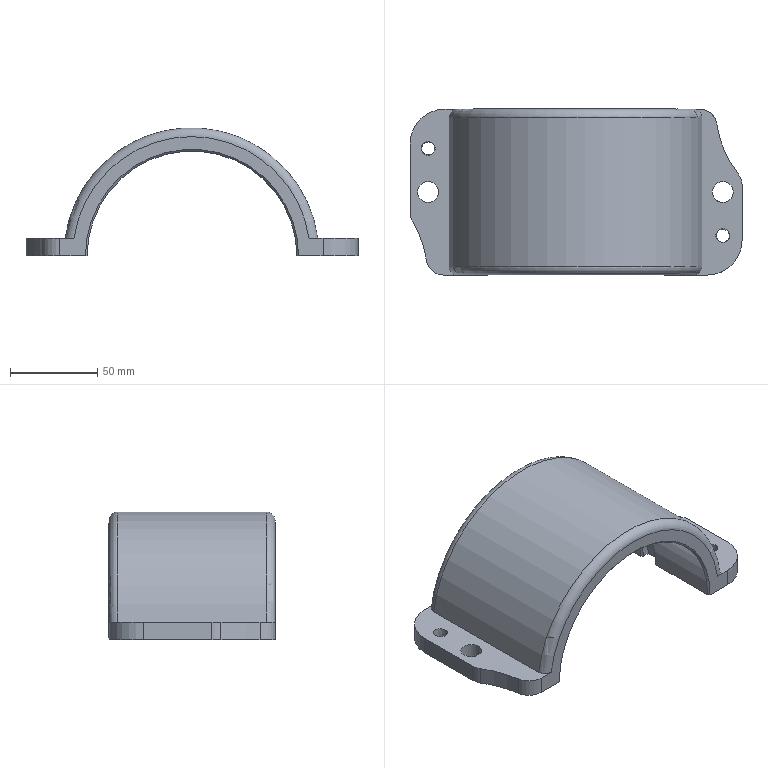Part | NX | features BREP 1, CHAMFER 1, DATUM_CSYS 1, DATUM_PLANE 1 | 1 solid | 32 faces | box 190 x 95 x 73.244 mm | volume 279574 mm3 | cylinder 14 | plane 10 | cone 6 | torus 2 | commonest cylinder face diameters 20 x4 120 x4 12 x2 40 x2 130 x1 146 x1
STEP:
#1=CARTESIAN_POINT('',(240.308,-695.5,40.));
#2=VERTEX_POINT('',#1);
#3=CARTESIAN_POINT('',(244.046,-695.5,40.));
#4=DIRECTION('',(0.,0.,-1.));
#5=DIRECTION('',(-1.,0.,0.));
#6=AXIS2_PLACEMENT_3D('',#3,#4,#5);
#7=CIRCLE('',#6,3.738);
#8=EDGE_CURVE('',#2,#2,#7,.F.);
#9=ORIENTED_EDGE('',*,*,#8,.T.);
#10=EDGE_LOOP('',(#9));
#11=FACE_BOUND('',#10,.T.);
#12=CARTESIAN_POINT('',(238.046,-670.5,40.));
#13=VERTEX_POINT('',#12);
#14=CARTESIAN_POINT('',(244.046,-670.5,40.));
#15=DIRECTION('',(0.,0.,-1.));
#16=DIRECTION('',(-1.,0.,0.));
#17=AXIS2_PLACEMENT_3D('',#14,#15,#16);
#18=CIRCLE('',#17,6.);
#19=EDGE_CURVE('',#13,#13,#18,.F.);
#20=ORIENTED_EDGE('',*,*,#19,.T.);
#21=EDGE_LOOP('',(#20));
#22=FACE_BOUND('',#21,.T.);
#23=CARTESIAN_POINT('',(220.,-624.,40.));
#24=VERTEX_POINT('',#23);
#25=CARTESIAN_POINT('',(220.,-663.,40.));
#26=VERTEX_POINT('',#25);
#27=CARTESIAN_POINT('',(220.,-611.,40.));
#28=DIRECTION('',(0.,-1.,0.));
#29=VECTOR('',#28,1000.);
#30=LINE('',#27,#29);
#31=EDGE_CURVE('',#24,#26,#30,.T.);
#32=ORIENTED_EDGE('',*,*,#31,.F.);
#33=CARTESIAN_POINT('',(221.,-623.,40.));
#34=VERTEX_POINT('',#33);
#35=CARTESIAN_POINT('',(160.,-684.,40.));
#36=DIRECTION('',(-0.7071,-0.7071,0.));
#37=VECTOR('',#36,1000.);
#38=LINE('',#35,#37);
#39=EDGE_CURVE('',#24,#34,#38,.F.);
#40=ORIENTED_EDGE('',*,*,#39,.T.);
#41=CARTESIAN_POINT('',(227.701,-623.,40.));
#42=VERTEX_POINT('',#41);
#43=CARTESIAN_POINT('',(85.,-623.,40.));
#44=DIRECTION('',(1.,0.,0.));
#45=VECTOR('',#44,1000.);
#46=LINE('',#43,#45);
#47=EDGE_CURVE('',#34,#42,#46,.T.);
#48=ORIENTED_EDGE('',*,*,#47,.T.);
#49=CARTESIAN_POINT('',(228.948,-623.158,40.));
#50=VERTEX_POINT('',#49);
#51=CARTESIAN_POINT('',(227.701,-623.,40.));
#52=CARTESIAN_POINT('',(228.123,-623.,40.));
#53=CARTESIAN_POINT('',(228.539,-623.053,40.));
#54=CARTESIAN_POINT('',(228.948,-623.158,40.));
#55=B_SPLINE_CURVE_WITH_KNOTS('',3,(#51,#52,#53,#54),.UNSPECIFIED.,.F.,.F.,(4,4),(0.,0.001257),.UNSPECIFIED.);
#56=EDGE_CURVE('',#42,#50,#55,.T.);
#57=ORIENTED_EDGE('',*,*,#56,.T.);
#58=CARTESIAN_POINT('',(240.615,-631.571,40.));
#59=VERTEX_POINT('',#58);
#60=CARTESIAN_POINT('',(230.718,-633.,40.));
#61=DIRECTION('',(0.,0.,-1.));
#62=DIRECTION('',(-1.,0.,0.));
#63=AXIS2_PLACEMENT_3D('',#60,#61,#62);
#64=CIRCLE('',#63,10.);
#65=EDGE_CURVE('',#50,#59,#64,.T.);
#66=ORIENTED_EDGE('',*,*,#65,.T.);
#67=CARTESIAN_POINT('',(252.857,-660.115,40.));
#68=VERTEX_POINT('',#67);
#69=CARTESIAN_POINT('',(300.,-623.,40.));
#70=DIRECTION('',(0.,0.,1.));
#71=DIRECTION('',(-1.,0.,0.));
#72=AXIS2_PLACEMENT_3D('',#69,#70,#71);
#73=CIRCLE('',#72,60.);
#74=EDGE_CURVE('',#59,#68,#73,.T.);
#75=ORIENTED_EDGE('',*,*,#74,.T.);
#76=CARTESIAN_POINT('',(255.,-666.301,40.));
#77=VERTEX_POINT('',#76);
#78=CARTESIAN_POINT('',(245.,-666.301,40.));
#79=DIRECTION('',(0.,0.,-1.));
#80=DIRECTION('',(-1.,0.,0.));
#81=AXIS2_PLACEMENT_3D('',#78,#79,#80);
#82=CIRCLE('',#81,10.);
#83=EDGE_CURVE('',#68,#77,#82,.T.);
#84=ORIENTED_EDGE('',*,*,#83,.T.);
#85=CARTESIAN_POINT('',(255.,-698.,40.));
#86=VERTEX_POINT('',#85);
#87=CARTESIAN_POINT('',(255.,-662.686,40.));
#88=DIRECTION('',(0.,-1.,0.));
#89=VECTOR('',#88,1000.);
#90=LINE('',#87,#89);
#91=EDGE_CURVE('',#77,#86,#90,.T.);
#92=ORIENTED_EDGE('',*,*,#91,.T.);
#93=CARTESIAN_POINT('',(235.,-718.,40.));
#94=VERTEX_POINT('',#93);
#95=CARTESIAN_POINT('',(235.,-698.,40.));
#96=DIRECTION('',(0.,0.,-1.));
#97=DIRECTION('',(-1.,0.,0.));
#98=AXIS2_PLACEMENT_3D('',#95,#96,#97);
#99=CIRCLE('',#98,20.);
#100=EDGE_CURVE('',#86,#94,#99,.T.);
#101=ORIENTED_EDGE('',*,*,#100,.T.);
#102=CARTESIAN_POINT('',(221.,-718.,40.));
#103=VERTEX_POINT('',#102);
#104=CARTESIAN_POINT('',(235.,-718.,40.));
#105=DIRECTION('',(-1.,0.,0.));
#106=VECTOR('',#105,1000.);
#107=LINE('',#104,#106);
#108=EDGE_CURVE('',#94,#103,#107,.T.);
#109=ORIENTED_EDGE('',*,*,#108,.T.);
#110=CARTESIAN_POINT('',(220.,-717.,40.));
#111=VERTEX_POINT('',#110);
#112=CARTESIAN_POINT('',(160.,-657.,40.));
#113=DIRECTION('',(0.7071,-0.7071,0.));
#114=VECTOR('',#113,1000.);
#115=LINE('',#112,#114);
#116=EDGE_CURVE('',#103,#111,#115,.F.);
#117=ORIENTED_EDGE('',*,*,#116,.T.);
#118=CARTESIAN_POINT('',(220.,-675.,40.));
#119=VERTEX_POINT('',#118);
#120=CARTESIAN_POINT('',(220.,-611.,40.));
#121=DIRECTION('',(0.,-1.,0.));
#122=VECTOR('',#121,1000.);
#123=LINE('',#120,#122);
#124=EDGE_CURVE('',#119,#111,#123,.T.);
#125=ORIENTED_EDGE('',*,*,#124,.F.);
#126=CARTESIAN_POINT('',(221.,-674.,40.));
#127=VERTEX_POINT('',#126);
#128=CARTESIAN_POINT('',(160.,-735.,40.));
#129=DIRECTION('',(-0.7071,-0.7071,0.));
#130=VECTOR('',#129,1000.);
#131=LINE('',#128,#130);
#132=EDGE_CURVE('',#119,#127,#131,.F.);
#133=ORIENTED_EDGE('',*,*,#132,.T.);
#134=CARTESIAN_POINT('',(225.,-674.,40.));
#135=VERTEX_POINT('',#134);
#136=CARTESIAN_POINT('',(85.,-674.,40.));
#137=DIRECTION('',(1.,0.,0.));
#138=VECTOR('',#137,1000.);
#139=LINE('',#136,#138);
#140=EDGE_CURVE('',#127,#135,#139,.T.);
#141=ORIENTED_EDGE('',*,*,#140,.T.);
#142=CARTESIAN_POINT('',(225.,-664.,40.));
#143=VERTEX_POINT('',#142);
#144=CARTESIAN_POINT('',(225.,-664.,40.));
#145=DIRECTION('',(0.,-1.,0.));
#146=VECTOR('',#145,1000.);
#147=LINE('',#144,#146);
#148=EDGE_CURVE('',#135,#143,#147,.F.);
#149=ORIENTED_EDGE('',*,*,#148,.T.);
#150=CARTESIAN_POINT('',(221.,-664.,40.));
#151=VERTEX_POINT('',#150);
#152=CARTESIAN_POINT('',(85.,-664.,40.));
#153=DIRECTION('',(1.,0.,0.));
#154=VECTOR('',#153,1000.);
#155=LINE('',#152,#154);
#156=EDGE_CURVE('',#151,#143,#155,.T.);
#157=ORIENTED_EDGE('',*,*,#156,.F.);
#158=CARTESIAN_POINT('',(160.,-603.,40.));
#159=DIRECTION('',(0.7071,-0.7071,0.));
#160=VECTOR('',#159,1000.);
#161=LINE('',#158,#160);
#162=EDGE_CURVE('',#151,#26,#161,.F.);
#163=ORIENTED_EDGE('',*,*,#162,.T.);
#164=EDGE_LOOP('',(#32,#40,#48,#57,#66,#75,#84,#92,#101,#109,#117,#125,#133,#141,#149,#157,#163));
#165=FACE_BOUND('',#164,.T.);
#166=CARTESIAN_POINT('',(85.,-643.,40.));
#167=DIRECTION('',(0.,0.,-1.));
#168=DIRECTION('',(-1.,0.,0.));
#169=AXIS2_PLACEMENT_3D('',#166,#167,#168);
#170=PLANE('',#169);
#171=ADVANCED_FACE('',(#11,#22,#165),#170,.T.);
#172=CARTESIAN_POINT('',(244.046,-691.5,50.));
#173=VERTEX_POINT('',#172);
#174=CARTESIAN_POINT('',(244.046,-695.5,50.));
#175=DIRECTION('',(0.,0.,-1.));
#176=DIRECTION('',(0.,1.,0.));
#177=AXIS2_PLACEMENT_3D('',#174,#175,#176);
#178=CIRCLE('',#177,4.);
#179=EDGE_CURVE('',#173,#173,#178,.T.);
#180=ORIENTED_EDGE('',*,*,#179,.T.);
#181=EDGE_LOOP('',(#180));
#182=FACE_BOUND('',#181,.T.);
#183=CARTESIAN_POINT('',(244.046,-664.5,50.));
#184=VERTEX_POINT('',#183);
#185=CARTESIAN_POINT('',(244.046,-670.5,50.));
#186=DIRECTION('',(0.,0.,-1.));
#187=DIRECTION('',(0.,1.,0.));
#188=AXIS2_PLACEMENT_3D('',#185,#186,#187);
#189=CIRCLE('',#188,6.);
#190=EDGE_CURVE('',#184,#184,#189,.T.);
#191=ORIENTED_EDGE('',*,*,#190,.T.);
#192=EDGE_LOOP('',(#191));
#193=FACE_BOUND('',#192,.T.);
#194=CARTESIAN_POINT('',(255.,-666.301,50.));
#195=VERTEX_POINT('',#194);
#196=CARTESIAN_POINT('',(255.,-698.,50.));
#197=VERTEX_POINT('',#196);
#198=CARTESIAN_POINT('',(255.,-662.686,50.));
#199=DIRECTION('',(0.,-1.,0.));
#200=VECTOR('',#199,1000.);
#201=LINE('',#198,#200);
#202=EDGE_CURVE('',#195,#197,#201,.T.);
#203=ORIENTED_EDGE('',*,*,#202,.F.);
#204=CARTESIAN_POINT('',(252.857,-660.115,50.));
#205=VERTEX_POINT('',#204);
#206=CARTESIAN_POINT('',(245.,-666.301,50.));
#207=DIRECTION('',(0.,0.,-1.));
#208=DIRECTION('',(-1.,0.,0.));
#209=AXIS2_PLACEMENT_3D('',#206,#207,#208);
#210=CIRCLE('',#209,10.);
#211=EDGE_CURVE('',#195,#205,#210,.F.);
#212=ORIENTED_EDGE('',*,*,#211,.T.);
#213=CARTESIAN_POINT('',(240.615,-631.571,50.));
#214=VERTEX_POINT('',#213);
#215=CARTESIAN_POINT('',(300.,-623.,50.));
#216=DIRECTION('',(0.,0.,1.));
#217=DIRECTION('',(-1.,0.,0.));
#218=AXIS2_PLACEMENT_3D('',#215,#216,#217);
#219=CIRCLE('',#218,60.);
#220=EDGE_CURVE('',#214,#205,#219,.T.);
#221=ORIENTED_EDGE('',*,*,#220,.F.);
#222=CARTESIAN_POINT('',(228.542,-623.24,50.));
#223=VERTEX_POINT('',#222);
#224=CARTESIAN_POINT('',(230.718,-633.,50.));
#225=DIRECTION('',(0.,0.,-1.));
#226=DIRECTION('',(-1.,0.,0.));
#227=AXIS2_PLACEMENT_3D('',#224,#225,#226);
#228=CIRCLE('',#227,10.);
#229=EDGE_CURVE('',#214,#223,#228,.F.);
#230=ORIENTED_EDGE('',*,*,#229,.T.);
#231=CARTESIAN_POINT('',(232.046,-628.,50.));
#232=VERTEX_POINT('',#231);
#233=CARTESIAN_POINT('',(228.542,-623.24,50.));
#234=CARTESIAN_POINT('',(229.555,-623.562,50.));
#235=CARTESIAN_POINT('',(231.34,-624.839,50.));
#236=CARTESIAN_POINT('',(232.046,-626.937,50.));
#237=CARTESIAN_POINT('',(232.046,-628.,50.));
#238=B_SPLINE_CURVE_WITH_KNOTS('',3,(#233,#234,#235,#236,#237),.UNSPECIFIED.,.F.,.F.,(4,1,4),(0.,0.003144,0.006288),.UNSPECIFIED.);
#239=EDGE_CURVE('',#223,#232,#238,.T.);
#240=ORIENTED_EDGE('',*,*,#239,.T.);
#241=CARTESIAN_POINT('',(232.046,-713.,50.));
#242=VERTEX_POINT('',#241);
#243=CARTESIAN_POINT('',(232.046,-623.,50.));
#244=DIRECTION('',(0.,-1.,0.));
#245=VECTOR('',#244,1000.);
#246=LINE('',#243,#245);
#247=EDGE_CURVE('',#232,#242,#246,.T.);
#248=ORIENTED_EDGE('',*,*,#247,.T.);
#249=CARTESIAN_POINT('',(226.998,-718.,50.));
#250=VERTEX_POINT('',#249);
#251=CARTESIAN_POINT('',(232.046,-713.,50.));
#252=CARTESIAN_POINT('',(232.046,-714.327,50.));
#253=CARTESIAN_POINT('',(230.936,-716.923,50.));
#254=CARTESIAN_POINT('',(228.324,-718.,50.));
#255=CARTESIAN_POINT('',(226.998,-718.,50.));
#256=B_SPLINE_CURVE_WITH_KNOTS('',3,(#251,#252,#253,#254,#255),.UNSPECIFIED.,.F.,.F.,(4,1,4),(0.,0.003925,0.007849),.UNSPECIFIED.);
#257=EDGE_CURVE('',#242,#250,#256,.T.);
#258=ORIENTED_EDGE('',*,*,#257,.T.);
#259=CARTESIAN_POINT('',(235.,-718.,50.));
#260=VERTEX_POINT('',#259);
#261=CARTESIAN_POINT('',(235.,-718.,50.));
#262=DIRECTION('',(-1.,0.,0.));
#263=VECTOR('',#262,1000.);
#264=LINE('',#261,#263);
#265=EDGE_CURVE('',#260,#250,#264,.T.);
#266=ORIENTED_EDGE('',*,*,#265,.F.);
#267=CARTESIAN_POINT('',(235.,-698.,50.));
#268=DIRECTION('',(0.,0.,-1.));
#269=DIRECTION('',(-1.,0.,0.));
#270=AXIS2_PLACEMENT_3D('',#267,#268,#269);
#271=CIRCLE('',#270,20.);
#272=EDGE_CURVE('',#197,#260,#271,.T.);
#273=ORIENTED_EDGE('',*,*,#272,.F.);
#274=EDGE_LOOP('',(#203,#212,#221,#230,#240,#248,#258,#266,#273));
#275=FACE_BOUND('',#274,.T.);
#276=CARTESIAN_POINT('',(85.,-643.,50.));
#277=DIRECTION('',(0.,0.,-1.));
#278=DIRECTION('',(-1.,0.,0.));
#279=AXIS2_PLACEMENT_3D('',#276,#277,#278);
#280=PLANE('',#279);
#281=ADVANCED_FACE('',(#182,#193,#275),#280,.F.);
#282=CARTESIAN_POINT('',(65.,-681.944,40.));
#283=VERTEX_POINT('',#282);
#284=CARTESIAN_POINT('',(65.,-643.,40.));
#285=VERTEX_POINT('',#284);
#286=CARTESIAN_POINT('',(65.,-684.834,40.));
#287=DIRECTION('',(0.,1.,0.));
#288=VECTOR('',#287,1000.);
#289=LINE('',#286,#288);
#290=EDGE_CURVE('',#283,#285,#289,.T.);
#291=ORIENTED_EDGE('',*,*,#290,.F.);
#292=CARTESIAN_POINT('',(65.,-681.944,50.));
#293=VERTEX_POINT('',#292);
#294=CARTESIAN_POINT('',(65.,-681.944,50.));
#295=DIRECTION('',(0.,0.,-1.));
#296=VECTOR('',#295,1000.);
#297=LINE('',#294,#296);
#298=EDGE_CURVE('',#283,#293,#297,.F.);
#299=ORIENTED_EDGE('',*,*,#298,.T.);
#300=CARTESIAN_POINT('',(65.,-643.,50.));
#301=VERTEX_POINT('',#300);
#302=CARTESIAN_POINT('',(65.,-684.834,50.));
#303=DIRECTION('',(0.,1.,0.));
#304=VECTOR('',#303,1000.);
#305=LINE('',#302,#304);
#306=EDGE_CURVE('',#293,#301,#305,.T.);
#307=ORIENTED_EDGE('',*,*,#306,.T.);
#308=CARTESIAN_POINT('',(65.,-643.,50.));
#309=DIRECTION('',(0.,0.,-1.));
#310=VECTOR('',#309,1000.);
#311=LINE('',#308,#310);
#312=EDGE_CURVE('',#301,#285,#311,.T.);
#313=ORIENTED_EDGE('',*,*,#312,.T.);
#314=EDGE_LOOP('',(#291,#299,#307,#313));
#315=FACE_BOUND('',#314,.T.);
#316=CARTESIAN_POINT('',(65.,-684.834,50.));
#317=DIRECTION('',(-1.,0.,0.));
#318=DIRECTION('',(0.,0.,1.));
#319=AXIS2_PLACEMENT_3D('',#316,#317,#318);
#320=PLANE('',#319);
#321=ADVANCED_FACE('',(#315),#320,.T.);
#322=CARTESIAN_POINT('',(85.,-623.,40.));
#323=VERTEX_POINT('',#322);
#324=CARTESIAN_POINT('',(85.,-643.,40.));
#325=DIRECTION('',(0.,0.,-1.));
#326=DIRECTION('',(-1.,0.,0.));
#327=AXIS2_PLACEMENT_3D('',#324,#325,#326);
#328=CIRCLE('',#327,20.);
#329=EDGE_CURVE('',#285,#323,#328,.T.);
#330=ORIENTED_EDGE('',*,*,#329,.F.);
#331=ORIENTED_EDGE('',*,*,#312,.F.);
#332=CARTESIAN_POINT('',(85.,-623.,50.));
#333=VERTEX_POINT('',#332);
#334=CARTESIAN_POINT('',(85.,-643.,50.));
#335=DIRECTION('',(0.,0.,-1.));
#336=DIRECTION('',(-1.,0.,0.));
#337=AXIS2_PLACEMENT_3D('',#334,#335,#336);
#338=CIRCLE('',#337,20.);
#339=EDGE_CURVE('',#301,#333,#338,.T.);
#340=ORIENTED_EDGE('',*,*,#339,.T.);
#341=CARTESIAN_POINT('',(85.,-623.,50.));
#342=DIRECTION('',(0.,0.,-1.));
#343=VECTOR('',#342,1000.);
#344=LINE('',#341,#343);
#345=EDGE_CURVE('',#333,#323,#344,.T.);
#346=ORIENTED_EDGE('',*,*,#345,.T.);
#347=EDGE_LOOP('',(#330,#331,#340,#346));
#348=FACE_BOUND('',#347,.T.);
#349=CARTESIAN_POINT('',(85.,-643.,50.));
#350=DIRECTION('',(0.,0.,-1.));
#351=DIRECTION('',(-1.,0.,0.));
#352=AXIS2_PLACEMENT_3D('',#349,#350,#351);
#353=CYLINDRICAL_SURFACE('',#352,20.);
#354=ADVANCED_FACE('',(#348),#353,.T.);
#355=ORIENTED_EDGE('',*,*,#47,.F.);
#356=CARTESIAN_POINT('',(99.,-623.,40.));
#357=VERTEX_POINT('',#356);
#358=CARTESIAN_POINT('',(160.,-623.,40.));
#359=DIRECTION('',(0.,1.,0.));
#360=DIRECTION('',(-1.,0.,0.));
#361=AXIS2_PLACEMENT_3D('',#358,#359,#360);
#362=CIRCLE('',#361,61.);
#363=EDGE_CURVE('',#34,#357,#362,.F.);
#364=ORIENTED_EDGE('',*,*,#363,.T.);
#365=CARTESIAN_POINT('',(85.,-623.,40.));
#366=DIRECTION('',(1.,0.,0.));
#367=VECTOR('',#366,1000.);
#368=LINE('',#365,#367);
#369=EDGE_CURVE('',#323,#357,#368,.T.);
#370=ORIENTED_EDGE('',*,*,#369,.F.);
#371=ORIENTED_EDGE('',*,*,#345,.F.);
#372=CARTESIAN_POINT('',(92.405,-623.,50.));
#373=VERTEX_POINT('',#372);
#374=CARTESIAN_POINT('',(85.,-623.,50.));
#375=DIRECTION('',(1.,0.,0.));
#376=VECTOR('',#375,1000.);
#377=LINE('',#374,#376);
#378=EDGE_CURVE('',#333,#373,#377,.T.);
#379=ORIENTED_EDGE('',*,*,#378,.T.);
#380=CARTESIAN_POINT('',(159.701,-623.,40.244));
#381=DIRECTION('',(0.,1.,0.));
#382=DIRECTION('',(-1.,0.,0.));
#383=AXIS2_PLACEMENT_3D('',#380,#381,#382);
#384=CIRCLE('',#383,68.);
#385=EDGE_CURVE('',#373,#42,#384,.T.);
#386=ORIENTED_EDGE('',*,*,#385,.T.);
#387=EDGE_LOOP('',(#355,#364,#370,#371,#379,#386));
#388=FACE_BOUND('',#387,.T.);
#389=CARTESIAN_POINT('',(85.,-623.,50.));
#390=DIRECTION('',(0.,1.,0.));
#391=DIRECTION('',(-1.,0.,0.));
#392=AXIS2_PLACEMENT_3D('',#389,#390,#391);
#393=PLANE('',#392);
#394=ADVANCED_FACE('',(#388),#393,.T.);
#395=ORIENTED_EDGE('',*,*,#220,.T.);
#396=CARTESIAN_POINT('',(252.857,-660.115,50.));
#397=DIRECTION('',(0.,0.,-1.));
#398=VECTOR('',#397,1000.);
#399=LINE('',#396,#398);
#400=EDGE_CURVE('',#205,#68,#399,.T.);
#401=ORIENTED_EDGE('',*,*,#400,.T.);
#402=ORIENTED_EDGE('',*,*,#74,.F.);
#403=CARTESIAN_POINT('',(240.615,-631.571,50.));
#404=DIRECTION('',(0.,0.,-1.));
#405=VECTOR('',#404,1000.);
#406=LINE('',#403,#405);
#407=EDGE_CURVE('',#59,#214,#406,.F.);
#408=ORIENTED_EDGE('',*,*,#407,.T.);
#409=EDGE_LOOP('',(#395,#401,#402,#408));
#410=FACE_BOUND('',#409,.T.);
#411=CARTESIAN_POINT('',(300.,-623.,50.));
#412=DIRECTION('',(0.,0.,-1.));
#413=DIRECTION('',(-1.,0.,0.));
#414=AXIS2_PLACEMENT_3D('',#411,#412,#413);
#415=CYLINDRICAL_SURFACE('',#414,60.);
#416=ADVANCED_FACE('',(#410),#415,.F.);
#417=ORIENTED_EDGE('',*,*,#91,.F.);
#418=CARTESIAN_POINT('',(255.,-666.301,50.));
#419=DIRECTION('',(0.,0.,-1.));
#420=VECTOR('',#419,1000.);
#421=LINE('',#418,#420);
#422=EDGE_CURVE('',#77,#195,#421,.F.);
#423=ORIENTED_EDGE('',*,*,#422,.T.);
#424=ORIENTED_EDGE('',*,*,#202,.T.);
#425=CARTESIAN_POINT('',(255.,-698.,50.));
#426=DIRECTION('',(0.,0.,-1.));
#427=VECTOR('',#426,1000.);
#428=LINE('',#425,#427);
#429=EDGE_CURVE('',#197,#86,#428,.T.);
#430=ORIENTED_EDGE('',*,*,#429,.T.);
#431=EDGE_LOOP('',(#417,#423,#424,#430));
#432=FACE_BOUND('',#431,.T.);
#433=CARTESIAN_POINT('',(255.,-662.686,50.));
#434=DIRECTION('',(1.,0.,0.));
#435=DIRECTION('',(0.,0.,-1.));
#436=AXIS2_PLACEMENT_3D('',#433,#434,#435);
#437=PLANE('',#436);
#438=ADVANCED_FACE('',(#432),#437,.T.);
#439=ORIENTED_EDGE('',*,*,#100,.F.);
#440=ORIENTED_EDGE('',*,*,#429,.F.);
#441=ORIENTED_EDGE('',*,*,#272,.T.);
#442=CARTESIAN_POINT('',(235.,-718.,50.));
#443=DIRECTION('',(0.,0.,-1.));
#444=VECTOR('',#443,1000.);
#445=LINE('',#442,#444);
#446=EDGE_CURVE('',#260,#94,#445,.T.);
#447=ORIENTED_EDGE('',*,*,#446,.T.);
#448=EDGE_LOOP('',(#439,#440,#441,#447));
#449=FACE_BOUND('',#448,.T.);
#450=CARTESIAN_POINT('',(235.,-698.,50.));
#451=DIRECTION('',(0.,0.,-1.));
#452=DIRECTION('',(-1.,0.,0.));
#453=AXIS2_PLACEMENT_3D('',#450,#451,#452);
#454=CYLINDRICAL_SURFACE('',#453,20.);
#455=ADVANCED_FACE('',(#449),#454,.T.);
#456=CARTESIAN_POINT('',(99.,-718.,40.));
#457=VERTEX_POINT('',#456);
#458=CARTESIAN_POINT('',(84.282,-718.,40.));
#459=VERTEX_POINT('',#458);
#460=CARTESIAN_POINT('',(235.,-718.,40.));
#461=DIRECTION('',(-1.,0.,0.));
#462=VECTOR('',#461,1000.);
#463=LINE('',#460,#462);
#464=EDGE_CURVE('',#457,#459,#463,.T.);
#465=ORIENTED_EDGE('',*,*,#464,.F.);
#466=CARTESIAN_POINT('',(160.,-718.,40.));
#467=DIRECTION('',(0.,-1.,0.));
#468=DIRECTION('',(0.,0.,-1.));
#469=AXIS2_PLACEMENT_3D('',#466,#467,#468);
#470=CIRCLE('',#469,61.);
#471=EDGE_CURVE('',#457,#103,#470,.F.);
#472=ORIENTED_EDGE('',*,*,#471,.T.);
#473=ORIENTED_EDGE('',*,*,#108,.F.);
#474=ORIENTED_EDGE('',*,*,#446,.F.);
#475=ORIENTED_EDGE('',*,*,#265,.T.);
#476=CARTESIAN_POINT('',(92.405,-718.,50.));
#477=VERTEX_POINT('',#476);
#478=CARTESIAN_POINT('',(159.701,-718.,40.244));
#479=DIRECTION('',(0.,-1.,0.));
#480=DIRECTION('',(0.,0.,-1.));
#481=AXIS2_PLACEMENT_3D('',#478,#479,#480);
#482=CIRCLE('',#481,68.);
#483=EDGE_CURVE('',#250,#477,#482,.T.);
#484=ORIENTED_EDGE('',*,*,#483,.T.);
#485=CARTESIAN_POINT('',(84.282,-718.,50.));
#486=VERTEX_POINT('',#485);
#487=CARTESIAN_POINT('',(235.,-718.,50.));
#488=DIRECTION('',(-1.,0.,0.));
#489=VECTOR('',#488,1000.);
#490=LINE('',#487,#489);
#491=EDGE_CURVE('',#477,#486,#490,.T.);
#492=ORIENTED_EDGE('',*,*,#491,.T.);
#493=CARTESIAN_POINT('',(84.282,-718.,50.));
#494=DIRECTION('',(0.,0.,-1.));
#495=VECTOR('',#494,1000.);
#496=LINE('',#493,#495);
#497=EDGE_CURVE('',#486,#459,#496,.T.);
#498=ORIENTED_EDGE('',*,*,#497,.T.);
#499=EDGE_LOOP('',(#465,#472,#473,#474,#475,#484,#492,#498));
#500=FACE_BOUND('',#499,.T.);
#501=CARTESIAN_POINT('',(235.,-718.,50.));
#502=DIRECTION('',(0.,-1.,0.));
#503=DIRECTION('',(0.,0.,-1.));
#504=AXIS2_PLACEMENT_3D('',#501,#502,#503);
#505=PLANE('',#504);
#506=ADVANCED_FACE('',(#500),#505,.T.);
#507=CARTESIAN_POINT('',(74.385,-709.429,50.));
#508=VERTEX_POINT('',#507);
#509=CARTESIAN_POINT('',(66.429,-687.095,50.));
#510=VERTEX_POINT('',#509);
#511=CARTESIAN_POINT('',(15.,-718.,50.));
#512=DIRECTION('',(0.,0.,1.));
#513=DIRECTION('',(-1.,0.,0.));
#514=AXIS2_PLACEMENT_3D('',#511,#512,#513);
#515=CIRCLE('',#514,60.);
#516=EDGE_CURVE('',#508,#510,#515,.T.);
#517=ORIENTED_EDGE('',*,*,#516,.T.);
#518=CARTESIAN_POINT('',(66.429,-687.095,40.));
#519=VERTEX_POINT('',#518);
#520=CARTESIAN_POINT('',(66.429,-687.095,50.));
#521=DIRECTION('',(0.,0.,-1.));
#522=VECTOR('',#521,1000.);
#523=LINE('',#520,#522);
#524=EDGE_CURVE('',#510,#519,#523,.T.);
#525=ORIENTED_EDGE('',*,*,#524,.T.);
#526=CARTESIAN_POINT('',(74.385,-709.429,40.));
#527=VERTEX_POINT('',#526);
#528=CARTESIAN_POINT('',(15.,-718.,40.));
#529=DIRECTION('',(0.,0.,1.));
#530=DIRECTION('',(-1.,0.,0.));
#531=AXIS2_PLACEMENT_3D('',#528,#529,#530);
#532=CIRCLE('',#531,60.);
#533=EDGE_CURVE('',#527,#519,#532,.T.);
#534=ORIENTED_EDGE('',*,*,#533,.F.);
#535=CARTESIAN_POINT('',(74.385,-709.429,50.));
#536=DIRECTION('',(0.,0.,-1.));
#537=VECTOR('',#536,1000.);
#538=LINE('',#535,#537);
#539=EDGE_CURVE('',#527,#508,#538,.F.);
#540=ORIENTED_EDGE('',*,*,#539,.T.);
#541=EDGE_LOOP('',(#517,#525,#534,#540));
#542=FACE_BOUND('',#541,.T.);
#543=CARTESIAN_POINT('',(15.,-718.,50.));
#544=DIRECTION('',(0.,0.,-1.));
#545=DIRECTION('',(-1.,0.,0.));
#546=AXIS2_PLACEMENT_3D('',#543,#544,#545);
#547=CYLINDRICAL_SURFACE('',#546,60.);
#548=ADVANCED_FACE('',(#542),#547,.F.);
#549=CARTESIAN_POINT('',(75.356,-641.5,50.));
#550=VERTEX_POINT('',#549);
#551=CARTESIAN_POINT('',(75.356,-645.5,50.));
#552=DIRECTION('',(0.,0.,1.));
#553=DIRECTION('',(0.,1.,0.));
#554=AXIS2_PLACEMENT_3D('',#551,#552,#553);
#555=CIRCLE('',#554,4.);
#556=EDGE_CURVE('',#550,#550,#555,.T.);
#557=ORIENTED_EDGE('',*,*,#556,.F.);
#558=EDGE_LOOP('',(#557));
#559=FACE_BOUND('',#558,.T.);
#560=CARTESIAN_POINT('',(75.356,-664.5,50.));
#561=VERTEX_POINT('',#560);
#562=CARTESIAN_POINT('',(75.356,-670.5,50.));
#563=DIRECTION('',(0.,0.,-1.));
#564=DIRECTION('',(0.,1.,0.));
#565=AXIS2_PLACEMENT_3D('',#562,#563,#564);
#566=CIRCLE('',#565,6.);
#567=EDGE_CURVE('',#561,#561,#566,.T.);
#568=ORIENTED_EDGE('',*,*,#567,.T.);
#569=EDGE_LOOP('',(#568));
#570=FACE_BOUND('',#569,.T.);
#571=ORIENTED_EDGE('',*,*,#306,.F.);
#572=CARTESIAN_POINT('',(75.,-681.944,50.));
#573=DIRECTION('',(0.,0.,-1.));
#574=DIRECTION('',(-1.,0.,0.));
#575=AXIS2_PLACEMENT_3D('',#572,#573,#574);
#576=CIRCLE('',#575,10.);
#577=EDGE_CURVE('',#293,#510,#576,.F.);
#578=ORIENTED_EDGE('',*,*,#577,.T.);
#579=ORIENTED_EDGE('',*,*,#516,.F.);
#580=CARTESIAN_POINT('',(84.282,-708.,50.));
#581=DIRECTION('',(0.,0.,-1.));
#582=DIRECTION('',(-1.,0.,0.));
#583=AXIS2_PLACEMENT_3D('',#580,#581,#582);
#584=CIRCLE('',#583,10.);
#585=EDGE_CURVE('',#508,#486,#584,.F.);
#586=ORIENTED_EDGE('',*,*,#585,.T.);
#587=ORIENTED_EDGE('',*,*,#491,.F.);
#588=CARTESIAN_POINT('',(87.356,-713.,50.));
#589=VERTEX_POINT('',#588);
#590=CARTESIAN_POINT('',(92.405,-718.,50.));
#591=CARTESIAN_POINT('',(91.078,-718.,50.));
#592=CARTESIAN_POINT('',(88.472,-716.928,50.));
#593=CARTESIAN_POINT('',(87.356,-714.327,50.));
#594=CARTESIAN_POINT('',(87.356,-713.,50.));
#595=B_SPLINE_CURVE_WITH_KNOTS('',3,(#590,#591,#592,#593,#594),.UNSPECIFIED.,.F.,.F.,(4,1,4),(0.,0.003925,0.007849),.UNSPECIFIED.);
#596=EDGE_CURVE('',#477,#589,#595,.T.);
#597=ORIENTED_EDGE('',*,*,#596,.T.);
#598=CARTESIAN_POINT('',(87.356,-628.,50.));
#599=VERTEX_POINT('',#598);
#600=CARTESIAN_POINT('',(87.356,-623.,50.));
#601=DIRECTION('',(0.,-1.,0.));
#602=VECTOR('',#601,1000.);
#603=LINE('',#600,#602);
#604=EDGE_CURVE('',#589,#599,#603,.F.);
#605=ORIENTED_EDGE('',*,*,#604,.T.);
#606=CARTESIAN_POINT('',(87.356,-628.,50.));
#607=CARTESIAN_POINT('',(87.356,-626.673,50.));
#608=CARTESIAN_POINT('',(88.467,-624.077,50.));
#609=CARTESIAN_POINT('',(91.078,-623.,50.));
#610=CARTESIAN_POINT('',(92.405,-623.,50.));
#611=B_SPLINE_CURVE_WITH_KNOTS('',3,(#606,#607,#608,#609,#610),.UNSPECIFIED.,.F.,.F.,(4,1,4),(0.,0.003925,0.007849),.UNSPECIFIED.);
#612=EDGE_CURVE('',#599,#373,#611,.T.);
#613=ORIENTED_EDGE('',*,*,#612,.T.);
#614=ORIENTED_EDGE('',*,*,#378,.F.);
#615=ORIENTED_EDGE('',*,*,#339,.F.);
#616=EDGE_LOOP('',(#571,#578,#579,#586,#587,#597,#605,#613,#614,#615));
#617=FACE_BOUND('',#616,.T.);
#618=CARTESIAN_POINT('',(85.,-643.,50.));
#619=DIRECTION('',(0.,0.,-1.));
#620=DIRECTION('',(-1.,0.,0.));
#621=AXIS2_PLACEMENT_3D('',#618,#619,#620);
#622=PLANE('',#621);
#623=ADVANCED_FACE('',(#559,#570,#617),#622,.F.);
#624=CARTESIAN_POINT('',(71.618,-645.5,40.));
#625=VERTEX_POINT('',#624);
#626=CARTESIAN_POINT('',(75.356,-645.5,40.));
#627=DIRECTION('',(0.,0.,-1.));
#628=DIRECTION('',(-1.,0.,0.));
#629=AXIS2_PLACEMENT_3D('',#626,#627,#628);
#630=CIRCLE('',#629,3.738);
#631=EDGE_CURVE('',#625,#625,#630,.T.);
#632=ORIENTED_EDGE('',*,*,#631,.F.);
#633=EDGE_LOOP('',(#632));
#634=FACE_BOUND('',#633,.T.);
#635=CARTESIAN_POINT('',(69.356,-670.5,40.));
#636=VERTEX_POINT('',#635);
#637=CARTESIAN_POINT('',(75.356,-670.5,40.));
#638=DIRECTION('',(0.,0.,-1.));
#639=DIRECTION('',(-1.,0.,0.));
#640=AXIS2_PLACEMENT_3D('',#637,#638,#639);
#641=CIRCLE('',#640,6.);
#642=EDGE_CURVE('',#636,#636,#641,.F.);
#643=ORIENTED_EDGE('',*,*,#642,.T.);
#644=EDGE_LOOP('',(#643));
#645=FACE_BOUND('',#644,.T.);
#646=ORIENTED_EDGE('',*,*,#369,.T.);
#647=CARTESIAN_POINT('',(100.,-624.,40.));
#648=VERTEX_POINT('',#647);
#649=CARTESIAN_POINT('',(160.,-684.,40.));
#650=DIRECTION('',(-0.7071,0.7071,0.));
#651=VECTOR('',#650,1000.);
#652=LINE('',#649,#651);
#653=EDGE_CURVE('',#357,#648,#652,.F.);
#654=ORIENTED_EDGE('',*,*,#653,.T.);
#655=CARTESIAN_POINT('',(100.,-663.,40.));
#656=VERTEX_POINT('',#655);
#657=CARTESIAN_POINT('',(100.,-611.,40.));
#658=DIRECTION('',(0.,-1.,0.));
#659=VECTOR('',#658,1000.);
#660=LINE('',#657,#659);
#661=EDGE_CURVE('',#656,#648,#660,.F.);
#662=ORIENTED_EDGE('',*,*,#661,.F.);
#663=CARTESIAN_POINT('',(99.,-664.,40.));
#664=VERTEX_POINT('',#663);
#665=CARTESIAN_POINT('',(160.,-603.,40.));
#666=DIRECTION('',(0.7071,0.7071,0.));
#667=VECTOR('',#666,1000.);
#668=LINE('',#665,#667);
#669=EDGE_CURVE('',#656,#664,#668,.F.);
#670=ORIENTED_EDGE('',*,*,#669,.T.);
#671=CARTESIAN_POINT('',(95.,-664.,40.));
#672=VERTEX_POINT('',#671);
#673=CARTESIAN_POINT('',(85.,-664.,40.));
#674=DIRECTION('',(1.,0.,0.));
#675=VECTOR('',#674,1000.);
#676=LINE('',#673,#675);
#677=EDGE_CURVE('',#672,#664,#676,.T.);
#678=ORIENTED_EDGE('',*,*,#677,.F.);
#679=CARTESIAN_POINT('',(95.,-674.,40.));
#680=VERTEX_POINT('',#679);
#681=CARTESIAN_POINT('',(95.,-664.,40.));
#682=DIRECTION('',(0.,-1.,0.));
#683=VECTOR('',#682,1000.);
#684=LINE('',#681,#683);
#685=EDGE_CURVE('',#672,#680,#684,.T.);
#686=ORIENTED_EDGE('',*,*,#685,.T.);
#687=CARTESIAN_POINT('',(99.,-674.,40.));
#688=VERTEX_POINT('',#687);
#689=CARTESIAN_POINT('',(85.,-674.,40.));
#690=DIRECTION('',(1.,0.,0.));
#691=VECTOR('',#690,1000.);
#692=LINE('',#689,#691);
#693=EDGE_CURVE('',#680,#688,#692,.T.);
#694=ORIENTED_EDGE('',*,*,#693,.T.);
#695=CARTESIAN_POINT('',(100.,-675.,40.));
#696=VERTEX_POINT('',#695);
#697=CARTESIAN_POINT('',(160.,-735.,40.));
#698=DIRECTION('',(-0.7071,0.7071,0.));
#699=VECTOR('',#698,1000.);
#700=LINE('',#697,#699);
#701=EDGE_CURVE('',#688,#696,#700,.F.);
#702=ORIENTED_EDGE('',*,*,#701,.T.);
#703=CARTESIAN_POINT('',(100.,-717.,40.));
#704=VERTEX_POINT('',#703);
#705=CARTESIAN_POINT('',(100.,-611.,40.));
#706=DIRECTION('',(0.,-1.,0.));
#707=VECTOR('',#706,1000.);
#708=LINE('',#705,#707);
#709=EDGE_CURVE('',#704,#696,#708,.F.);
#710=ORIENTED_EDGE('',*,*,#709,.F.);
#711=CARTESIAN_POINT('',(160.,-657.,40.));
#712=DIRECTION('',(0.7071,0.7071,0.));
#713=VECTOR('',#712,1000.);
#714=LINE('',#711,#713);
#715=EDGE_CURVE('',#704,#457,#714,.F.);
#716=ORIENTED_EDGE('',*,*,#715,.T.);
#717=ORIENTED_EDGE('',*,*,#464,.T.);
#718=CARTESIAN_POINT('',(84.282,-708.,40.));
#719=DIRECTION('',(0.,0.,-1.));
#720=DIRECTION('',(-1.,0.,0.));
#721=AXIS2_PLACEMENT_3D('',#718,#719,#720);
#722=CIRCLE('',#721,10.);
#723=EDGE_CURVE('',#459,#527,#722,.T.);
#724=ORIENTED_EDGE('',*,*,#723,.T.);
#725=ORIENTED_EDGE('',*,*,#533,.T.);
#726=CARTESIAN_POINT('',(75.,-681.944,40.));
#727=DIRECTION('',(0.,0.,-1.));
#728=DIRECTION('',(-1.,0.,0.));
#729=AXIS2_PLACEMENT_3D('',#726,#727,#728);
#730=CIRCLE('',#729,10.);
#731=EDGE_CURVE('',#519,#283,#730,.T.);
#732=ORIENTED_EDGE('',*,*,#731,.T.);
#733=ORIENTED_EDGE('',*,*,#290,.T.);
#734=ORIENTED_EDGE('',*,*,#329,.T.);
#735=EDGE_LOOP('',(#646,#654,#662,#670,#678,#686,#694,#702,#710,#716,#717,#724,#725,#732,#733,#734));
#736=FACE_BOUND('',#735,.T.);
#737=CARTESIAN_POINT('',(85.,-643.,40.));
#738=DIRECTION('',(0.,0.,-1.));
#739=DIRECTION('',(-1.,0.,0.));
#740=AXIS2_PLACEMENT_3D('',#737,#738,#739);
#741=PLANE('',#740);
#742=ADVANCED_FACE('',(#634,#645,#736),#741,.T.);
#743=ORIENTED_EDGE('',*,*,#604,.F.);
#744=CARTESIAN_POINT('',(159.701,-713.,40.244));
#745=DIRECTION('',(0.,-1.,0.));
#746=DIRECTION('',(0.,0.,-1.));
#747=AXIS2_PLACEMENT_3D('',#744,#745,#746);
#748=CIRCLE('',#747,73.);
#749=EDGE_CURVE('',#589,#242,#748,.F.);
#750=ORIENTED_EDGE('',*,*,#749,.T.);
#751=ORIENTED_EDGE('',*,*,#247,.F.);
#752=CARTESIAN_POINT('',(159.701,-628.,40.244));
#753=DIRECTION('',(0.,1.,0.));
#754=DIRECTION('',(-1.,0.,0.));
#755=AXIS2_PLACEMENT_3D('',#752,#753,#754);
#756=CIRCLE('',#755,73.);
#757=EDGE_CURVE('',#232,#599,#756,.F.);
#758=ORIENTED_EDGE('',*,*,#757,.T.);
#759=EDGE_LOOP('',(#743,#750,#751,#758));
#760=FACE_BOUND('',#759,.T.);
#761=CARTESIAN_POINT('',(159.701,-623.,40.244));
#762=DIRECTION('',(0.,-1.,0.));
#763=DIRECTION('',(0.,0.,-1.));
#764=AXIS2_PLACEMENT_3D('',#761,#762,#763);
#765=CYLINDRICAL_SURFACE('',#764,73.);
#766=ADVANCED_FACE('',(#760),#765,.T.);
#767=CARTESIAN_POINT('',(160.,-674.,40.));
#768=DIRECTION('',(0.,1.,0.));
#769=DIRECTION('',(1.,0.,0.));
#770=AXIS2_PLACEMENT_3D('',#767,#768,#769);
#771=CIRCLE('',#770,65.);
#772=EDGE_CURVE('',#135,#680,#771,.F.);
#773=ORIENTED_EDGE('',*,*,#772,.T.);
#774=ORIENTED_EDGE('',*,*,#685,.F.);
#775=CARTESIAN_POINT('',(160.,-664.,40.));
#776=DIRECTION('',(0.,1.,0.));
#777=DIRECTION('',(1.,0.,0.));
#778=AXIS2_PLACEMENT_3D('',#775,#776,#777);
#779=CIRCLE('',#778,65.);
#780=EDGE_CURVE('',#143,#672,#779,.F.);
#781=ORIENTED_EDGE('',*,*,#780,.F.);
#782=ORIENTED_EDGE('',*,*,#148,.F.);
#783=EDGE_LOOP('',(#773,#774,#781,#782));
#784=FACE_BOUND('',#783,.T.);
#785=CARTESIAN_POINT('',(160.,-664.,40.));
#786=DIRECTION('',(0.,-1.,0.));
#787=DIRECTION('',(0.,0.,-1.));
#788=AXIS2_PLACEMENT_3D('',#785,#786,#787);
#789=CYLINDRICAL_SURFACE('',#788,65.);
#790=ADVANCED_FACE('',(#784),#789,.F.);
#791=ORIENTED_EDGE('',*,*,#677,.T.);
#792=CARTESIAN_POINT('',(160.,-664.,40.));
#793=DIRECTION('',(0.,1.,0.));
#794=DIRECTION('',(0.,0.,1.));
#795=AXIS2_PLACEMENT_3D('',#792,#793,#794);
#796=CIRCLE('',#795,61.);
#797=EDGE_CURVE('',#664,#151,#796,.T.);
#798=ORIENTED_EDGE('',*,*,#797,.T.);
#799=ORIENTED_EDGE('',*,*,#156,.T.);
#800=ORIENTED_EDGE('',*,*,#780,.T.);
#801=EDGE_LOOP('',(#791,#798,#799,#800));
#802=FACE_BOUND('',#801,.T.);
#803=CARTESIAN_POINT('',(160.,-664.,40.));
#804=DIRECTION('',(0.,1.,0.));
#805=DIRECTION('',(0.,0.,1.));
#806=AXIS2_PLACEMENT_3D('',#803,#804,#805);
#807=PLANE('',#806);
#808=ADVANCED_FACE('',(#802),#807,.F.);
#809=ORIENTED_EDGE('',*,*,#140,.F.);
#810=CARTESIAN_POINT('',(160.,-674.,40.));
#811=DIRECTION('',(0.,1.,0.));
#812=DIRECTION('',(0.,0.,1.));
#813=AXIS2_PLACEMENT_3D('',#810,#811,#812);
#814=CIRCLE('',#813,61.);
#815=EDGE_CURVE('',#127,#688,#814,.F.);
#816=ORIENTED_EDGE('',*,*,#815,.T.);
#817=ORIENTED_EDGE('',*,*,#693,.F.);
#818=ORIENTED_EDGE('',*,*,#772,.F.);
#819=EDGE_LOOP('',(#809,#816,#817,#818));
#820=FACE_BOUND('',#819,.T.);
#821=CARTESIAN_POINT('',(160.,-674.,40.));
#822=DIRECTION('',(0.,1.,0.));
#823=DIRECTION('',(0.,0.,1.));
#824=AXIS2_PLACEMENT_3D('',#821,#822,#823);
#825=PLANE('',#824);
#826=ADVANCED_FACE('',(#820),#825,.T.);
#827=ORIENTED_EDGE('',*,*,#124,.T.);
#828=CARTESIAN_POINT('',(160.,-717.,40.));
#829=DIRECTION('',(0.,-1.,0.));
#830=DIRECTION('',(0.,0.,-1.));
#831=AXIS2_PLACEMENT_3D('',#828,#829,#830);
#832=CIRCLE('',#831,60.);
#833=EDGE_CURVE('',#111,#704,#832,.T.);
#834=ORIENTED_EDGE('',*,*,#833,.T.);
#835=ORIENTED_EDGE('',*,*,#709,.T.);
#836=CARTESIAN_POINT('',(160.,-675.,40.));
#837=DIRECTION('',(0.,1.,0.));
#838=DIRECTION('',(0.,0.,1.));
#839=AXIS2_PLACEMENT_3D('',#836,#837,#838);
#840=CIRCLE('',#839,60.);
#841=EDGE_CURVE('',#696,#119,#840,.T.);
#842=ORIENTED_EDGE('',*,*,#841,.T.);
#843=EDGE_LOOP('',(#827,#834,#835,#842));
#844=FACE_BOUND('',#843,.T.);
#845=CARTESIAN_POINT('',(160.,-611.,40.));
#846=DIRECTION('',(0.,-1.,0.));
#847=DIRECTION('',(0.,0.,-1.));
#848=AXIS2_PLACEMENT_3D('',#845,#846,#847);
#849=CYLINDRICAL_SURFACE('',#848,60.);
#850=ADVANCED_FACE('',(#844),#849,.F.);
#851=ORIENTED_EDGE('',*,*,#661,.T.);
#852=CARTESIAN_POINT('',(160.,-624.,40.));
#853=DIRECTION('',(0.,1.,0.));
#854=DIRECTION('',(0.,0.,1.));
#855=AXIS2_PLACEMENT_3D('',#852,#853,#854);
#856=CIRCLE('',#855,60.);
#857=EDGE_CURVE('',#648,#24,#856,.T.);
#858=ORIENTED_EDGE('',*,*,#857,.T.);
#859=ORIENTED_EDGE('',*,*,#31,.T.);
#860=CARTESIAN_POINT('',(160.,-663.,40.));
#861=DIRECTION('',(0.,1.,0.));
#862=DIRECTION('',(0.,0.,1.));
#863=AXIS2_PLACEMENT_3D('',#860,#861,#862);
#864=CIRCLE('',#863,60.);
#865=EDGE_CURVE('',#26,#656,#864,.F.);
#866=ORIENTED_EDGE('',*,*,#865,.T.);
#867=EDGE_LOOP('',(#851,#858,#859,#866));
#868=FACE_BOUND('',#867,.T.);
#869=CARTESIAN_POINT('',(160.,-611.,40.));
#870=DIRECTION('',(0.,-1.,0.));
#871=DIRECTION('',(0.,0.,-1.));
#872=AXIS2_PLACEMENT_3D('',#869,#870,#871);
#873=CYLINDRICAL_SURFACE('',#872,60.);
#874=ADVANCED_FACE('',(#868),#873,.F.);
#875=ORIENTED_EDGE('',*,*,#701,.F.);
#876=ORIENTED_EDGE('',*,*,#815,.F.);
#877=ORIENTED_EDGE('',*,*,#132,.F.);
#878=ORIENTED_EDGE('',*,*,#841,.F.);
#879=EDGE_LOOP('',(#875,#876,#877,#878));
#880=FACE_BOUND('',#879,.T.);
#881=CARTESIAN_POINT('',(160.,-675.,40.));
#882=DIRECTION('',(0.,1.,0.));
#883=DIRECTION('',(0.,0.,1.));
#884=AXIS2_PLACEMENT_3D('',#881,#882,#883);
#885=CONICAL_SURFACE('',#884,60.,0.7854);
#886=ADVANCED_FACE('',(#880),#885,.F.);
#887=ORIENTED_EDGE('',*,*,#669,.F.);
#888=ORIENTED_EDGE('',*,*,#865,.F.);
#889=ORIENTED_EDGE('',*,*,#162,.F.);
#890=ORIENTED_EDGE('',*,*,#797,.F.);
#891=EDGE_LOOP('',(#887,#888,#889,#890));
#892=FACE_BOUND('',#891,.T.);
#893=CARTESIAN_POINT('',(160.,-664.,40.));
#894=DIRECTION('',(0.,-1.,0.));
#895=DIRECTION('',(0.,0.,-1.));
#896=AXIS2_PLACEMENT_3D('',#893,#894,#895);
#897=CONICAL_SURFACE('',#896,61.,0.7854);
#898=ADVANCED_FACE('',(#892),#897,.F.);
#899=ORIENTED_EDGE('',*,*,#642,.F.);
#900=EDGE_LOOP('',(#899));
#901=FACE_BOUND('',#900,.T.);
#902=ORIENTED_EDGE('',*,*,#567,.F.);
#903=EDGE_LOOP('',(#902));
#904=FACE_BOUND('',#903,.T.);
#905=CARTESIAN_POINT('',(75.356,-670.5,-220.));
#906=DIRECTION('',(0.,0.,1.));
#907=DIRECTION('',(1.,0.,0.));
#908=AXIS2_PLACEMENT_3D('',#905,#906,#907);
#909=CYLINDRICAL_SURFACE('',#908,6.);
#910=ADVANCED_FACE('',(#901,#904),#909,.F.);
#911=ORIENTED_EDGE('',*,*,#19,.F.);
#912=EDGE_LOOP('',(#911));
#913=FACE_BOUND('',#912,.T.);
#914=ORIENTED_EDGE('',*,*,#190,.F.);
#915=EDGE_LOOP('',(#914));
#916=FACE_BOUND('',#915,.T.);
#917=CARTESIAN_POINT('',(244.046,-670.5,-220.));
#918=DIRECTION('',(0.,0.,1.));
#919=DIRECTION('',(1.,0.,0.));
#920=AXIS2_PLACEMENT_3D('',#917,#918,#919);
#921=CYLINDRICAL_SURFACE('',#920,6.);
#922=ADVANCED_FACE('',(#913,#916),#921,.F.);
#923=ORIENTED_EDGE('',*,*,#8,.F.);
#924=EDGE_LOOP('',(#923));
#925=FACE_BOUND('',#924,.T.);
#926=ORIENTED_EDGE('',*,*,#179,.F.);
#927=EDGE_LOOP('',(#926));
#928=FACE_BOUND('',#927,.T.);
#929=CARTESIAN_POINT('',(244.046,-695.5,50.));
#930=DIRECTION('',(0.,0.,1.));
#931=DIRECTION('',(0.,1.,0.));
#932=AXIS2_PLACEMENT_3D('',#929,#930,#931);
#933=CONICAL_SURFACE('',#932,4.,0.02618);
#934=ADVANCED_FACE('',(#925,#928),#933,.F.);
#935=ORIENTED_EDGE('',*,*,#631,.T.);
#936=EDGE_LOOP('',(#935));
#937=FACE_BOUND('',#936,.T.);
#938=ORIENTED_EDGE('',*,*,#556,.T.);
#939=EDGE_LOOP('',(#938));
#940=FACE_BOUND('',#939,.T.);
#941=CARTESIAN_POINT('',(75.356,-645.5,50.));
#942=DIRECTION('',(0.,0.,1.));
#943=DIRECTION('',(0.,1.,0.));
#944=AXIS2_PLACEMENT_3D('',#941,#942,#943);
#945=CONICAL_SURFACE('',#944,4.,0.02618);
#946=ADVANCED_FACE('',(#937,#940),#945,.F.);
#947=ORIENTED_EDGE('',*,*,#211,.F.);
#948=ORIENTED_EDGE('',*,*,#422,.F.);
#949=ORIENTED_EDGE('',*,*,#83,.F.);
#950=ORIENTED_EDGE('',*,*,#400,.F.);
#951=EDGE_LOOP('',(#947,#948,#949,#950));
#952=FACE_BOUND('',#951,.T.);
#953=CARTESIAN_POINT('',(245.,-666.301,50.));
#954=DIRECTION('',(0.,0.,-1.));
#955=DIRECTION('',(-1.,0.,0.));
#956=AXIS2_PLACEMENT_3D('',#953,#954,#955);
#957=CYLINDRICAL_SURFACE('',#956,10.);
#958=ADVANCED_FACE('',(#952),#957,.T.);
#959=ORIENTED_EDGE('',*,*,#577,.F.);
#960=ORIENTED_EDGE('',*,*,#298,.F.);
#961=ORIENTED_EDGE('',*,*,#731,.F.);
#962=ORIENTED_EDGE('',*,*,#524,.F.);
#963=EDGE_LOOP('',(#959,#960,#961,#962));
#964=FACE_BOUND('',#963,.T.);
#965=CARTESIAN_POINT('',(75.,-681.944,50.));
#966=DIRECTION('',(0.,0.,-1.));
#967=DIRECTION('',(-1.,0.,0.));
#968=AXIS2_PLACEMENT_3D('',#965,#966,#967);
#969=CYLINDRICAL_SURFACE('',#968,10.);
#970=ADVANCED_FACE('',(#964),#969,.T.);
#971=ORIENTED_EDGE('',*,*,#585,.F.);
#972=ORIENTED_EDGE('',*,*,#539,.F.);
#973=ORIENTED_EDGE('',*,*,#723,.F.);
#974=ORIENTED_EDGE('',*,*,#497,.F.);
#975=EDGE_LOOP('',(#971,#972,#973,#974));
#976=FACE_BOUND('',#975,.T.);
#977=CARTESIAN_POINT('',(84.282,-708.,50.));
#978=DIRECTION('',(0.,0.,-1.));
#979=DIRECTION('',(-1.,0.,0.));
#980=AXIS2_PLACEMENT_3D('',#977,#978,#979);
#981=CYLINDRICAL_SURFACE('',#980,10.);
#982=ADVANCED_FACE('',(#976),#981,.T.);
#983=ORIENTED_EDGE('',*,*,#229,.F.);
#984=ORIENTED_EDGE('',*,*,#407,.F.);
#985=ORIENTED_EDGE('',*,*,#65,.F.);
#986=CARTESIAN_POINT('',(228.948,-623.158,40.));
#987=CARTESIAN_POINT('',(228.954,-623.157,43.339));
#988=CARTESIAN_POINT('',(228.82,-623.178,46.673));
#989=CARTESIAN_POINT('',(228.542,-623.24,50.));
#990=B_SPLINE_CURVE_WITH_KNOTS('',3,(#986,#987,#988,#989),.UNSPECIFIED.,.F.,.F.,(4,4),(0.,0.01001),.UNSPECIFIED.);
#991=EDGE_CURVE('',#50,#223,#990,.T.);
#992=ORIENTED_EDGE('',*,*,#991,.T.);
#993=EDGE_LOOP('',(#983,#984,#985,#992));
#994=FACE_BOUND('',#993,.T.);
#995=CARTESIAN_POINT('',(230.718,-633.,50.));
#996=DIRECTION('',(0.,0.,-1.));
#997=DIRECTION('',(-1.,0.,0.));
#998=AXIS2_PLACEMENT_3D('',#995,#996,#997);
#999=CYLINDRICAL_SURFACE('',#998,10.);
#1000=ADVANCED_FACE('',(#994),#999,.T.);
#1001=ORIENTED_EDGE('',*,*,#257,.F.);
#1002=ORIENTED_EDGE('',*,*,#749,.F.);
#1003=ORIENTED_EDGE('',*,*,#596,.F.);
#1004=ORIENTED_EDGE('',*,*,#483,.F.);
#1005=EDGE_LOOP('',(#1001,#1002,#1003,#1004));
#1006=FACE_BOUND('',#1005,.T.);
#1007=CARTESIAN_POINT('',(159.701,-713.,40.244));
#1008=DIRECTION('',(0.,-1.,0.));
#1009=DIRECTION('',(0.,0.,-1.));
#1010=AXIS2_PLACEMENT_3D('',#1007,#1008,#1009);
#1011=TOROIDAL_SURFACE('',#1010,68.,5.);
#1012=ADVANCED_FACE('',(#1006),#1011,.T.);
#1013=ORIENTED_EDGE('',*,*,#56,.F.);
#1014=ORIENTED_EDGE('',*,*,#385,.F.);
#1015=ORIENTED_EDGE('',*,*,#612,.F.);
#1016=ORIENTED_EDGE('',*,*,#757,.F.);
#1017=ORIENTED_EDGE('',*,*,#239,.F.);
#1018=ORIENTED_EDGE('',*,*,#991,.F.);
#1019=EDGE_LOOP('',(#1013,#1014,#1015,#1016,#1017,#1018));
#1020=FACE_BOUND('',#1019,.T.);
#1021=CARTESIAN_POINT('',(159.701,-628.,40.244));
#1022=DIRECTION('',(0.,1.,0.));
#1023=DIRECTION('',(-1.,0.,0.));
#1024=AXIS2_PLACEMENT_3D('',#1021,#1022,#1023);
#1025=TOROIDAL_SURFACE('',#1024,68.,5.);
#1026=ADVANCED_FACE('',(#1020),#1025,.T.);
#1027=ORIENTED_EDGE('',*,*,#653,.F.);
#1028=ORIENTED_EDGE('',*,*,#363,.F.);
#1029=ORIENTED_EDGE('',*,*,#39,.F.);
#1030=ORIENTED_EDGE('',*,*,#857,.F.);
#1031=EDGE_LOOP('',(#1027,#1028,#1029,#1030));
#1032=FACE_BOUND('',#1031,.T.);
#1033=CARTESIAN_POINT('',(160.,-624.,40.));
#1034=DIRECTION('',(0.,1.,0.));
#1035=DIRECTION('',(0.,0.,1.));
#1036=AXIS2_PLACEMENT_3D('',#1033,#1034,#1035);
#1037=CONICAL_SURFACE('',#1036,60.,0.7854);
#1038=ADVANCED_FACE('',(#1032),#1037,.F.);
#1039=ORIENTED_EDGE('',*,*,#116,.F.);
#1040=ORIENTED_EDGE('',*,*,#471,.F.);
#1041=ORIENTED_EDGE('',*,*,#715,.F.);
#1042=ORIENTED_EDGE('',*,*,#833,.F.);
#1043=EDGE_LOOP('',(#1039,#1040,#1041,#1042));
#1044=FACE_BOUND('',#1043,.T.);
#1045=CARTESIAN_POINT('',(160.,-717.,40.));
#1046=DIRECTION('',(0.,-1.,0.));
#1047=DIRECTION('',(0.,0.,-1.));
#1048=AXIS2_PLACEMENT_3D('',#1045,#1046,#1047);
#1049=CONICAL_SURFACE('',#1048,60.,0.7854);
#1050=ADVANCED_FACE('',(#1044),#1049,.F.);
#1051=CLOSED_SHELL('',(#171,#281,#321,#354,#394,#416,#438,#455,#506,#548,#623,#742,#766,#790,#808,#826,#850,#874,#886,#898,#910,#922,#934,#946,#958,#970,#982,#1000,#1012,#1026,#1038,#1050));
#1052=MANIFOLD_SOLID_BREP('',#1051);
#1053=(LENGTH_UNIT()NAMED_UNIT(*)SI_UNIT(.MILLI.,.METRE.));
#1054=UNCERTAINTY_MEASURE_WITH_UNIT(LENGTH_MEASURE(0.0508),#1053,'','');
#1055=(NAMED_UNIT(*)PLANE_ANGLE_UNIT()SI_UNIT($,.RADIAN.));
#1056=(NAMED_UNIT(*)SI_UNIT($,.STERADIAN.)SOLID_ANGLE_UNIT());
#1057=(GEOMETRIC_REPRESENTATION_CONTEXT(3)GLOBAL_UNCERTAINTY_ASSIGNED_CONTEXT((#1054))GLOBAL_UNIT_ASSIGNED_CONTEXT((#1053,#1055,#1056))REPRESENTATION_CONTEXT('',''));
#1058=ADVANCED_BREP_SHAPE_REPRESENTATION('',(#1052),#1057);